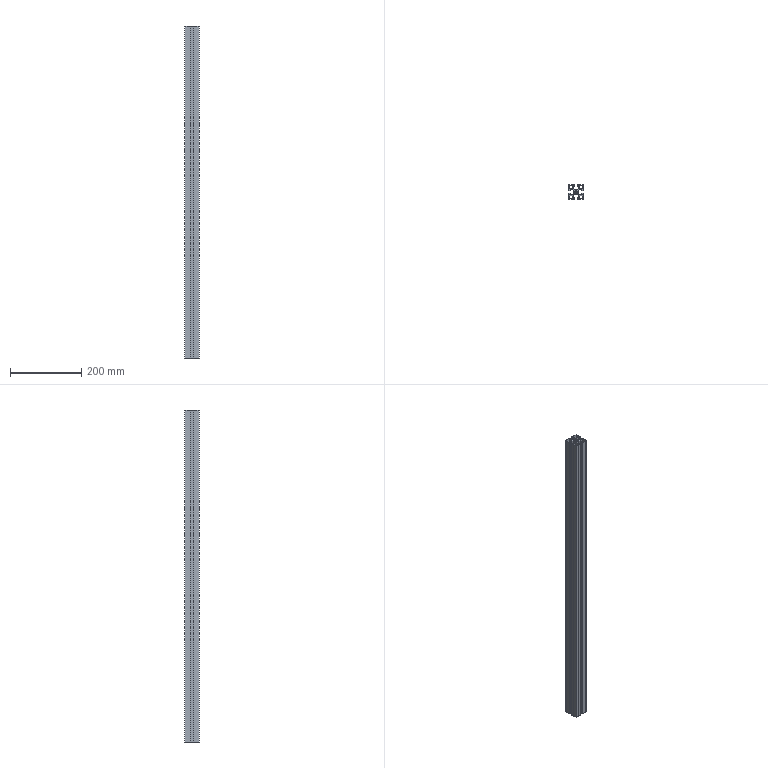Part | STEP file | 40C-2 | 1 solid | 64 faces | box 40 x 40 x 930 mm | volume 488011 mm3 | plane 62 | cylinder 2 | commonest cylinder face diameters 6.8 x2